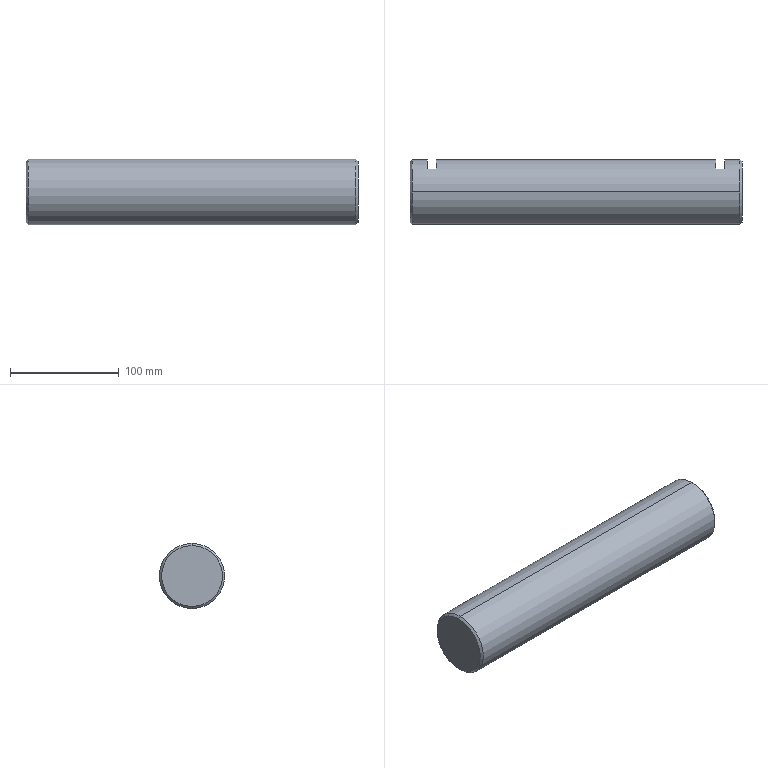Part | STEP file | 04-Driven shaft 1 | 1 solid | 14 faces | box 305 x 60 x 60 mm | volume 857375 mm3 | plane 8 | cone 4 | cylinder 2 | commonest cylinder face diameters 60 x2
STEP:
#1=CARTESIAN_POINT('',(0.,0.,0.));
#2=DIRECTION('',(0.,0.,1.));
#3=DIRECTION('',(1.,0.,0.));
#4=AXIS2_PLACEMENT_3D('',#1,#2,#3);
#5=CARTESIAN_POINT('',(305.,0.,-28.));
#6=VERTEX_POINT('',#5);
#7=CARTESIAN_POINT('',(305.,0.,28.));
#8=VERTEX_POINT('',#7);
#9=CARTESIAN_POINT('',(305.,0.,0.));
#10=DIRECTION('',(1.,0.,0.));
#11=DIRECTION('',(0.,0.,1.));
#12=AXIS2_PLACEMENT_3D('',#9,#10,#11);
#13=CIRCLE('',#12,28.);
#14=CARTESIAN_POINT('',(303.,0.,0.));
#15=DIRECTION('',(-1.,0.,0.));
#16=DIRECTION('',(0.,0.,1.));
#17=AXIS2_PLACEMENT_3D('',#14,#15,#16);
#18=CONICAL_SURFACE('',#17,30.,0.7854);
#19=CARTESIAN_POINT('',(6.283,-2.));
#20=DIRECTION('',(-1.,0.));
#21=VECTOR('',#20,1.);
#22=LINE('',#19,#21);
#23=(GEOMETRIC_REPRESENTATION_CONTEXT(2)PARAMETRIC_REPRESENTATION_CONTEXT()REPRESENTATION_CONTEXT('',''));
#24=DEFINITIONAL_REPRESENTATION('',(#22),#23);
#25=PCURVE('',#18,#24);
#26=CARTESIAN_POINT('',(305.,30.,0.));
#27=DIRECTION('',(-1.,0.,0.));
#28=DIRECTION('',(0.,0.,1.));
#29=AXIS2_PLACEMENT_3D('',#26,#27,#28);
#30=PLANE('',#29);
#31=CARTESIAN_POINT('',(28.,-30.));
#32=CARTESIAN_POINT('',(28.,-78.497));
#33=CARTESIAN_POINT('',(-14.,-54.249));
#34=CARTESIAN_POINT('',(-56.,-30.));
#35=CARTESIAN_POINT('',(-14.,-5.751));
#36=CARTESIAN_POINT('',(28.,18.497));
#37=CARTESIAN_POINT('',(28.,-30.));
#38=(BOUNDED_CURVE()B_SPLINE_CURVE(2,(#31,#32,#33,#34,#35,#36,#37),.UNSPECIFIED.,.T.,.F.)B_SPLINE_CURVE_WITH_KNOTS((1,2,2,2,2,1),(-2.094,0.,2.094,4.189,6.283,8.378),.UNSPECIFIED.)CURVE()GEOMETRIC_REPRESENTATION_ITEM()RATIONAL_B_SPLINE_CURVE((1.,0.5,1.,0.5,1.,0.5,1.))REPRESENTATION_ITEM(''));
#39=(GEOMETRIC_REPRESENTATION_CONTEXT(2)PARAMETRIC_REPRESENTATION_CONTEXT()REPRESENTATION_CONTEXT('',''));
#40=DEFINITIONAL_REPRESENTATION('',(#38),#39);
#41=PCURVE('',#30,#40);
#42=SURFACE_CURVE('',#13,(#25,#41),.PCURVE_S1.);
#43=EDGE_CURVE('',#6,#8,#42,.T.);
#44=ORIENTED_EDGE('',*,*,#43,.F.);
#45=CARTESIAN_POINT('',(303.,0.,-30.));
#46=VERTEX_POINT('',#45);
#47=CARTESIAN_POINT('',(303.,0.,-30.));
#48=DIRECTION('',(-0.7071,0.,-0.7071));
#49=VECTOR('',#48,1.);
#50=LINE('',#47,#49);
#51=CARTESIAN_POINT('',(3.142,0.));
#52=DIRECTION('',(0.,1.));
#53=VECTOR('',#52,1.);
#54=LINE('',#51,#53);
#55=(GEOMETRIC_REPRESENTATION_CONTEXT(2)PARAMETRIC_REPRESENTATION_CONTEXT()REPRESENTATION_CONTEXT('',''));
#56=DEFINITIONAL_REPRESENTATION('',(#54),#55);
#57=PCURVE('',#18,#56);
#58=CARTESIAN_POINT('',(303.,0.,0.));
#59=DIRECTION('',(-1.,0.,0.));
#60=DIRECTION('',(0.,0.,1.));
#61=AXIS2_PLACEMENT_3D('',#58,#59,#60);
#62=CONICAL_SURFACE('',#61,30.,0.7854);
#63=CARTESIAN_POINT('',(3.142,0.));
#64=DIRECTION('',(0.,1.));
#65=VECTOR('',#64,1.);
#66=LINE('',#63,#65);
#67=(GEOMETRIC_REPRESENTATION_CONTEXT(2)PARAMETRIC_REPRESENTATION_CONTEXT()REPRESENTATION_CONTEXT('',''));
#68=DEFINITIONAL_REPRESENTATION('',(#66),#67);
#69=PCURVE('',#62,#68);
#70=SURFACE_CURVE('',#50,(#57,#69),.PCURVE_S1.);
#71=EDGE_CURVE('',#6,#46,#70,.T.);
#72=ORIENTED_EDGE('',*,*,#71,.T.);
#73=CARTESIAN_POINT('',(303.,0.,30.));
#74=VERTEX_POINT('',#73);
#75=CARTESIAN_POINT('',(303.,0.,0.));
#76=DIRECTION('',(-1.,0.,0.));
#77=DIRECTION('',(0.,0.,1.));
#78=AXIS2_PLACEMENT_3D('',#75,#76,#77);
#79=CIRCLE('',#78,30.);
#80=CARTESIAN_POINT('',(0.,0.));
#81=DIRECTION('',(1.,0.));
#82=VECTOR('',#81,1.);
#83=LINE('',#80,#82);
#84=(GEOMETRIC_REPRESENTATION_CONTEXT(2)PARAMETRIC_REPRESENTATION_CONTEXT()REPRESENTATION_CONTEXT('',''));
#85=DEFINITIONAL_REPRESENTATION('',(#83),#84);
#86=PCURVE('',#18,#85);
#87=CARTESIAN_POINT('',(0.,0.,0.));
#88=DIRECTION('',(-1.,0.,0.));
#89=DIRECTION('',(0.,0.,1.));
#90=AXIS2_PLACEMENT_3D('',#87,#88,#89);
#91=CYLINDRICAL_SURFACE('',#90,30.);
#92=CARTESIAN_POINT('',(0.,-303.));
#93=DIRECTION('',(1.,0.));
#94=VECTOR('',#93,1.);
#95=LINE('',#92,#94);
#96=(GEOMETRIC_REPRESENTATION_CONTEXT(2)PARAMETRIC_REPRESENTATION_CONTEXT()REPRESENTATION_CONTEXT('',''));
#97=DEFINITIONAL_REPRESENTATION('',(#95),#96);
#98=PCURVE('',#91,#97);
#99=SURFACE_CURVE('',#79,(#86,#98),.PCURVE_S1.);
#100=EDGE_CURVE('',#74,#46,#99,.T.);
#101=ORIENTED_EDGE('',*,*,#100,.F.);
#102=CARTESIAN_POINT('',(303.,0.,30.));
#103=DIRECTION('',(-0.7071,0.,0.7071));
#104=VECTOR('',#103,1.);
#105=LINE('',#102,#104);
#106=CARTESIAN_POINT('',(0.,0.));
#107=DIRECTION('',(0.,1.));
#108=VECTOR('',#107,1.);
#109=LINE('',#106,#108);
#110=(GEOMETRIC_REPRESENTATION_CONTEXT(2)PARAMETRIC_REPRESENTATION_CONTEXT()REPRESENTATION_CONTEXT('',''));
#111=DEFINITIONAL_REPRESENTATION('',(#109),#110);
#112=PCURVE('',#18,#111);
#113=CARTESIAN_POINT('',(6.283,0.));
#114=DIRECTION('',(0.,1.));
#115=VECTOR('',#114,1.);
#116=LINE('',#113,#115);
#117=(GEOMETRIC_REPRESENTATION_CONTEXT(2)PARAMETRIC_REPRESENTATION_CONTEXT()REPRESENTATION_CONTEXT('',''));
#118=DEFINITIONAL_REPRESENTATION('',(#116),#117);
#119=PCURVE('',#62,#118);
#120=SURFACE_CURVE('',#105,(#112,#119),.PCURVE_S1.);
#121=EDGE_CURVE('',#8,#74,#120,.T.);
#122=ORIENTED_EDGE('',*,*,#121,.F.);
#123=EDGE_LOOP('',(#44,#72,#101,#122));
#124=FACE_BOUND('',#123,.T.);
#125=ADVANCED_FACE('',(#124),#18,.T.);
#126=CARTESIAN_POINT('',(0.,0.,28.));
#127=VERTEX_POINT('',#126);
#128=CARTESIAN_POINT('',(0.,0.,-28.));
#129=VERTEX_POINT('',#128);
#130=CARTESIAN_POINT('',(0.,0.,0.));
#131=DIRECTION('',(-1.,0.,0.));
#132=DIRECTION('',(0.,0.,-1.));
#133=AXIS2_PLACEMENT_3D('',#130,#131,#132);
#134=CIRCLE('',#133,28.);
#135=CARTESIAN_POINT('',(0.,0.,0.));
#136=DIRECTION('',(1.,0.,0.));
#137=DIRECTION('',(0.,0.,-1.));
#138=AXIS2_PLACEMENT_3D('',#135,#136,#137);
#139=CONICAL_SURFACE('',#138,28.,0.7854);
#140=CARTESIAN_POINT('',(6.283,0.));
#141=DIRECTION('',(-1.,0.));
#142=VECTOR('',#141,1.);
#143=LINE('',#140,#142);
#144=(GEOMETRIC_REPRESENTATION_CONTEXT(2)PARAMETRIC_REPRESENTATION_CONTEXT()REPRESENTATION_CONTEXT('',''));
#145=DEFINITIONAL_REPRESENTATION('',(#143),#144);
#146=PCURVE('',#139,#145);
#147=CARTESIAN_POINT('',(0.,0.,0.));
#148=DIRECTION('',(1.,0.,0.));
#149=DIRECTION('',(0.,0.,-1.));
#150=AXIS2_PLACEMENT_3D('',#147,#148,#149);
#151=PLANE('',#150);
#152=CARTESIAN_POINT('',(28.,0.));
#153=CARTESIAN_POINT('',(28.,-48.497));
#154=CARTESIAN_POINT('',(-14.,-24.249));
#155=CARTESIAN_POINT('',(-56.,0.));
#156=CARTESIAN_POINT('',(-14.,24.249));
#157=CARTESIAN_POINT('',(28.,48.497));
#158=CARTESIAN_POINT('',(28.,0.));
#159=(BOUNDED_CURVE()B_SPLINE_CURVE(2,(#152,#153,#154,#155,#156,#157,#158),.UNSPECIFIED.,.T.,.F.)B_SPLINE_CURVE_WITH_KNOTS((1,2,2,2,2,1),(-2.094,0.,2.094,4.189,6.283,8.378),.UNSPECIFIED.)CURVE()GEOMETRIC_REPRESENTATION_ITEM()RATIONAL_B_SPLINE_CURVE((1.,0.5,1.,0.5,1.,0.5,1.))REPRESENTATION_ITEM(''));
#160=(GEOMETRIC_REPRESENTATION_CONTEXT(2)PARAMETRIC_REPRESENTATION_CONTEXT()REPRESENTATION_CONTEXT('',''));
#161=DEFINITIONAL_REPRESENTATION('',(#159),#160);
#162=PCURVE('',#151,#161);
#163=SURFACE_CURVE('',#134,(#146,#162),.PCURVE_S1.);
#164=EDGE_CURVE('',#127,#129,#163,.T.);
#165=ORIENTED_EDGE('',*,*,#164,.F.);
#166=CARTESIAN_POINT('',(2.,0.,30.));
#167=VERTEX_POINT('',#166);
#168=CARTESIAN_POINT('',(0.,0.,28.));
#169=DIRECTION('',(0.7071,0.,0.7071));
#170=VECTOR('',#169,1.);
#171=LINE('',#168,#170);
#172=CARTESIAN_POINT('',(3.142,0.));
#173=DIRECTION('',(0.,1.));
#174=VECTOR('',#173,1.);
#175=LINE('',#172,#174);
#176=(GEOMETRIC_REPRESENTATION_CONTEXT(2)PARAMETRIC_REPRESENTATION_CONTEXT()REPRESENTATION_CONTEXT('',''));
#177=DEFINITIONAL_REPRESENTATION('',(#175),#176);
#178=PCURVE('',#139,#177);
#179=CARTESIAN_POINT('',(0.,0.,0.));
#180=DIRECTION('',(1.,0.,0.));
#181=DIRECTION('',(0.,0.,-1.));
#182=AXIS2_PLACEMENT_3D('',#179,#180,#181);
#183=CONICAL_SURFACE('',#182,28.,0.7854);
#184=CARTESIAN_POINT('',(3.142,0.));
#185=DIRECTION('',(0.,1.));
#186=VECTOR('',#185,1.);
#187=LINE('',#184,#186);
#188=(GEOMETRIC_REPRESENTATION_CONTEXT(2)PARAMETRIC_REPRESENTATION_CONTEXT()REPRESENTATION_CONTEXT('',''));
#189=DEFINITIONAL_REPRESENTATION('',(#187),#188);
#190=PCURVE('',#183,#189);
#191=SURFACE_CURVE('',#171,(#178,#190),.PCURVE_S1.);
#192=EDGE_CURVE('',#127,#167,#191,.T.);
#193=ORIENTED_EDGE('',*,*,#192,.T.);
#194=CARTESIAN_POINT('',(2.,0.,-30.));
#195=VERTEX_POINT('',#194);
#196=CARTESIAN_POINT('',(2.,0.,0.));
#197=DIRECTION('',(1.,0.,0.));
#198=DIRECTION('',(0.,0.,-1.));
#199=AXIS2_PLACEMENT_3D('',#196,#197,#198);
#200=CIRCLE('',#199,30.);
#201=CARTESIAN_POINT('',(0.,2.));
#202=DIRECTION('',(1.,0.));
#203=VECTOR('',#202,1.);
#204=LINE('',#201,#203);
#205=(GEOMETRIC_REPRESENTATION_CONTEXT(2)PARAMETRIC_REPRESENTATION_CONTEXT()REPRESENTATION_CONTEXT('',''));
#206=DEFINITIONAL_REPRESENTATION('',(#204),#205);
#207=PCURVE('',#139,#206);
#208=CARTESIAN_POINT('',(3.142,-2.));
#209=DIRECTION('',(-1.,0.));
#210=VECTOR('',#209,1.);
#211=LINE('',#208,#210);
#212=(GEOMETRIC_REPRESENTATION_CONTEXT(2)PARAMETRIC_REPRESENTATION_CONTEXT()REPRESENTATION_CONTEXT('',''));
#213=DEFINITIONAL_REPRESENTATION('',(#211),#212);
#214=PCURVE('',#91,#213);
#215=SURFACE_CURVE('',#200,(#207,#214),.PCURVE_S1.);
#216=EDGE_CURVE('',#195,#167,#215,.T.);
#217=ORIENTED_EDGE('',*,*,#216,.F.);
#218=CARTESIAN_POINT('',(0.,0.,-28.));
#219=DIRECTION('',(0.7071,0.,-0.7071));
#220=VECTOR('',#219,1.);
#221=LINE('',#218,#220);
#222=CARTESIAN_POINT('',(0.,0.));
#223=DIRECTION('',(0.,1.));
#224=VECTOR('',#223,1.);
#225=LINE('',#222,#224);
#226=(GEOMETRIC_REPRESENTATION_CONTEXT(2)PARAMETRIC_REPRESENTATION_CONTEXT()REPRESENTATION_CONTEXT('',''));
#227=DEFINITIONAL_REPRESENTATION('',(#225),#226);
#228=PCURVE('',#139,#227);
#229=CARTESIAN_POINT('',(6.283,0.));
#230=DIRECTION('',(0.,1.));
#231=VECTOR('',#230,1.);
#232=LINE('',#229,#231);
#233=(GEOMETRIC_REPRESENTATION_CONTEXT(2)PARAMETRIC_REPRESENTATION_CONTEXT()REPRESENTATION_CONTEXT('',''));
#234=DEFINITIONAL_REPRESENTATION('',(#232),#233);
#235=PCURVE('',#183,#234);
#236=SURFACE_CURVE('',#221,(#228,#235),.PCURVE_S1.);
#237=EDGE_CURVE('',#129,#195,#236,.T.);
#238=ORIENTED_EDGE('',*,*,#237,.F.);
#239=EDGE_LOOP('',(#165,#193,#217,#238));
#240=FACE_BOUND('',#239,.T.);
#241=ADVANCED_FACE('',(#240),#139,.T.);
#242=CARTESIAN_POINT('',(24.,21.,-21.424));
#243=VERTEX_POINT('',#242);
#244=CARTESIAN_POINT('',(16.,21.,-21.424));
#245=VERTEX_POINT('',#244);
#246=CARTESIAN_POINT('',(0.,21.,-21.424));
#247=DIRECTION('',(-1.,0.,0.));
#248=VECTOR('',#247,1.);
#249=LINE('',#246,#248);
#250=CARTESIAN_POINT('',(2.366,0.));
#251=DIRECTION('',(0.,1.));
#252=VECTOR('',#251,1.);
#253=LINE('',#250,#252);
#254=(GEOMETRIC_REPRESENTATION_CONTEXT(2)PARAMETRIC_REPRESENTATION_CONTEXT()REPRESENTATION_CONTEXT('',''));
#255=DEFINITIONAL_REPRESENTATION('',(#253),#254);
#256=PCURVE('',#91,#255);
#257=CARTESIAN_POINT('',(0.,21.,0.));
#258=DIRECTION('',(0.,1.,0.));
#259=DIRECTION('',(0.,0.,1.));
#260=AXIS2_PLACEMENT_3D('',#257,#258,#259);
#261=PLANE('',#260);
#262=CARTESIAN_POINT('',(-21.424,0.));
#263=DIRECTION('',(0.,-1.));
#264=VECTOR('',#263,1.);
#265=LINE('',#262,#264);
#266=(GEOMETRIC_REPRESENTATION_CONTEXT(2)PARAMETRIC_REPRESENTATION_CONTEXT()REPRESENTATION_CONTEXT('',''));
#267=DEFINITIONAL_REPRESENTATION('',(#265),#266);
#268=PCURVE('',#261,#267);
#269=SURFACE_CURVE('',#249,(#256,#268),.PCURVE_S1.);
#270=EDGE_CURVE('',#243,#245,#269,.T.);
#271=ORIENTED_EDGE('',*,*,#270,.F.);
#272=CARTESIAN_POINT('',(24.,21.,21.424));
#273=VERTEX_POINT('',#272);
#274=CARTESIAN_POINT('',(24.,0.,0.));
#275=DIRECTION('',(-1.,0.,0.));
#276=DIRECTION('',(0.,0.,1.));
#277=AXIS2_PLACEMENT_3D('',#274,#275,#276);
#278=CIRCLE('',#277,30.);
#279=CARTESIAN_POINT('',(0.,-24.));
#280=DIRECTION('',(1.,0.));
#281=VECTOR('',#280,1.);
#282=LINE('',#279,#281);
#283=(GEOMETRIC_REPRESENTATION_CONTEXT(2)PARAMETRIC_REPRESENTATION_CONTEXT()REPRESENTATION_CONTEXT('',''));
#284=DEFINITIONAL_REPRESENTATION('',(#282),#283);
#285=PCURVE('',#91,#284);
#286=CARTESIAN_POINT('',(24.,31.,-45.622));
#287=DIRECTION('',(-1.,0.,0.));
#288=DIRECTION('',(0.,0.,1.));
#289=AXIS2_PLACEMENT_3D('',#286,#287,#288);
#290=PLANE('',#289);
#291=CARTESIAN_POINT('',(45.622,-31.));
#292=DIRECTION('',(1.,0.));
#293=AXIS2_PLACEMENT_2D('',#291,#292);
#294=CIRCLE('',#293,30.);
#295=(GEOMETRIC_REPRESENTATION_CONTEXT(2)PARAMETRIC_REPRESENTATION_CONTEXT()REPRESENTATION_CONTEXT('',''));
#296=DEFINITIONAL_REPRESENTATION('',(#294),#295);
#297=PCURVE('',#290,#296);
#298=SURFACE_CURVE('',#278,(#285,#297),.PCURVE_S1.);
#299=EDGE_CURVE('',#273,#243,#298,.T.);
#300=ORIENTED_EDGE('',*,*,#299,.F.);
#301=CARTESIAN_POINT('',(16.,21.,21.424));
#302=VERTEX_POINT('',#301);
#303=CARTESIAN_POINT('',(0.,21.,21.424));
#304=DIRECTION('',(1.,0.,0.));
#305=VECTOR('',#304,1.);
#306=LINE('',#303,#305);
#307=CARTESIAN_POINT('',(0.7754,0.));
#308=DIRECTION('',(0.,-1.));
#309=VECTOR('',#308,1.);
#310=LINE('',#307,#309);
#311=(GEOMETRIC_REPRESENTATION_CONTEXT(2)PARAMETRIC_REPRESENTATION_CONTEXT()REPRESENTATION_CONTEXT('',''));
#312=DEFINITIONAL_REPRESENTATION('',(#310),#311);
#313=PCURVE('',#91,#312);
#314=CARTESIAN_POINT('',(21.424,0.));
#315=DIRECTION('',(0.,1.));
#316=VECTOR('',#315,1.);
#317=LINE('',#314,#316);
#318=(GEOMETRIC_REPRESENTATION_CONTEXT(2)PARAMETRIC_REPRESENTATION_CONTEXT()REPRESENTATION_CONTEXT('',''));
#319=DEFINITIONAL_REPRESENTATION('',(#317),#318);
#320=PCURVE('',#261,#319);
#321=SURFACE_CURVE('',#306,(#313,#320),.PCURVE_S1.);
#322=EDGE_CURVE('',#302,#273,#321,.T.);
#323=ORIENTED_EDGE('',*,*,#322,.F.);
#324=CARTESIAN_POINT('',(16.,0.,0.));
#325=DIRECTION('',(1.,0.,0.));
#326=DIRECTION('',(0.,0.,-1.));
#327=AXIS2_PLACEMENT_3D('',#324,#325,#326);
#328=CIRCLE('',#327,30.);
#329=CARTESIAN_POINT('',(3.142,-16.));
#330=DIRECTION('',(-1.,0.));
#331=VECTOR('',#330,1.);
#332=LINE('',#329,#331);
#333=(GEOMETRIC_REPRESENTATION_CONTEXT(2)PARAMETRIC_REPRESENTATION_CONTEXT()REPRESENTATION_CONTEXT('',''));
#334=DEFINITIONAL_REPRESENTATION('',(#332),#333);
#335=PCURVE('',#91,#334);
#336=CARTESIAN_POINT('',(16.,31.,-45.622));
#337=DIRECTION('',(1.,0.,0.));
#338=DIRECTION('',(0.,0.,-1.));
#339=AXIS2_PLACEMENT_3D('',#336,#337,#338);
#340=PLANE('',#339);
#341=CARTESIAN_POINT('',(-45.622,-31.));
#342=DIRECTION('',(1.,0.));
#343=AXIS2_PLACEMENT_2D('',#341,#342);
#344=CIRCLE('',#343,30.);
#345=(GEOMETRIC_REPRESENTATION_CONTEXT(2)PARAMETRIC_REPRESENTATION_CONTEXT()REPRESENTATION_CONTEXT('',''));
#346=DEFINITIONAL_REPRESENTATION('',(#344),#345);
#347=PCURVE('',#340,#346);
#348=SURFACE_CURVE('',#328,(#335,#347),.PCURVE_S1.);
#349=EDGE_CURVE('',#245,#302,#348,.T.);
#350=ORIENTED_EDGE('',*,*,#349,.F.);
#351=EDGE_LOOP('',(#271,#300,#323,#350));
#352=FACE_BOUND('',#351,.T.);
#353=CARTESIAN_POINT('',(289.,21.,-21.424));
#354=VERTEX_POINT('',#353);
#355=CARTESIAN_POINT('',(281.,21.,-21.424));
#356=VERTEX_POINT('',#355);
#357=CARTESIAN_POINT('',(0.,21.,-21.424));
#358=DIRECTION('',(-1.,0.,0.));
#359=VECTOR('',#358,1.);
#360=LINE('',#357,#359);
#361=CARTESIAN_POINT('',(2.366,0.));
#362=DIRECTION('',(0.,1.));
#363=VECTOR('',#362,1.);
#364=LINE('',#361,#363);
#365=(GEOMETRIC_REPRESENTATION_CONTEXT(2)PARAMETRIC_REPRESENTATION_CONTEXT()REPRESENTATION_CONTEXT('',''));
#366=DEFINITIONAL_REPRESENTATION('',(#364),#365);
#367=PCURVE('',#91,#366);
#368=CARTESIAN_POINT('',(0.,21.,0.));
#369=DIRECTION('',(0.,1.,0.));
#370=DIRECTION('',(0.,0.,1.));
#371=AXIS2_PLACEMENT_3D('',#368,#369,#370);
#372=PLANE('',#371);
#373=CARTESIAN_POINT('',(-21.424,0.));
#374=DIRECTION('',(0.,-1.));
#375=VECTOR('',#374,1.);
#376=LINE('',#373,#375);
#377=(GEOMETRIC_REPRESENTATION_CONTEXT(2)PARAMETRIC_REPRESENTATION_CONTEXT()REPRESENTATION_CONTEXT('',''));
#378=DEFINITIONAL_REPRESENTATION('',(#376),#377);
#379=PCURVE('',#372,#378);
#380=SURFACE_CURVE('',#360,(#367,#379),.PCURVE_S1.);
#381=EDGE_CURVE('',#354,#356,#380,.T.);
#382=ORIENTED_EDGE('',*,*,#381,.F.);
#383=CARTESIAN_POINT('',(289.,21.,21.424));
#384=VERTEX_POINT('',#383);
#385=CARTESIAN_POINT('',(289.,0.,0.));
#386=DIRECTION('',(-1.,0.,0.));
#387=DIRECTION('',(0.,0.,1.));
#388=AXIS2_PLACEMENT_3D('',#385,#386,#387);
#389=CIRCLE('',#388,30.);
#390=CARTESIAN_POINT('',(0.,-289.));
#391=DIRECTION('',(1.,0.));
#392=VECTOR('',#391,1.);
#393=LINE('',#390,#392);
#394=(GEOMETRIC_REPRESENTATION_CONTEXT(2)PARAMETRIC_REPRESENTATION_CONTEXT()REPRESENTATION_CONTEXT('',''));
#395=DEFINITIONAL_REPRESENTATION('',(#393),#394);
#396=PCURVE('',#91,#395);
#397=CARTESIAN_POINT('',(289.,31.,-54.746));
#398=DIRECTION('',(-1.,0.,0.));
#399=DIRECTION('',(0.,0.,1.));
#400=AXIS2_PLACEMENT_3D('',#397,#398,#399);
#401=PLANE('',#400);
#402=CARTESIAN_POINT('',(54.746,-31.));
#403=DIRECTION('',(1.,0.));
#404=AXIS2_PLACEMENT_2D('',#402,#403);
#405=CIRCLE('',#404,30.);
#406=(GEOMETRIC_REPRESENTATION_CONTEXT(2)PARAMETRIC_REPRESENTATION_CONTEXT()REPRESENTATION_CONTEXT('',''));
#407=DEFINITIONAL_REPRESENTATION('',(#405),#406);
#408=PCURVE('',#401,#407);
#409=SURFACE_CURVE('',#389,(#396,#408),.PCURVE_S1.);
#410=EDGE_CURVE('',#384,#354,#409,.T.);
#411=ORIENTED_EDGE('',*,*,#410,.F.);
#412=CARTESIAN_POINT('',(281.,21.,21.424));
#413=VERTEX_POINT('',#412);
#414=CARTESIAN_POINT('',(0.,21.,21.424));
#415=DIRECTION('',(1.,0.,0.));
#416=VECTOR('',#415,1.);
#417=LINE('',#414,#416);
#418=CARTESIAN_POINT('',(0.7754,0.));
#419=DIRECTION('',(0.,-1.));
#420=VECTOR('',#419,1.);
#421=LINE('',#418,#420);
#422=(GEOMETRIC_REPRESENTATION_CONTEXT(2)PARAMETRIC_REPRESENTATION_CONTEXT()REPRESENTATION_CONTEXT('',''));
#423=DEFINITIONAL_REPRESENTATION('',(#421),#422);
#424=PCURVE('',#91,#423);
#425=CARTESIAN_POINT('',(21.424,0.));
#426=DIRECTION('',(0.,1.));
#427=VECTOR('',#426,1.);
#428=LINE('',#425,#427);
#429=(GEOMETRIC_REPRESENTATION_CONTEXT(2)PARAMETRIC_REPRESENTATION_CONTEXT()REPRESENTATION_CONTEXT('',''));
#430=DEFINITIONAL_REPRESENTATION('',(#428),#429);
#431=PCURVE('',#372,#430);
#432=SURFACE_CURVE('',#417,(#424,#431),.PCURVE_S1.);
#433=EDGE_CURVE('',#413,#384,#432,.T.);
#434=ORIENTED_EDGE('',*,*,#433,.F.);
#435=CARTESIAN_POINT('',(281.,0.,0.));
#436=DIRECTION('',(1.,0.,0.));
#437=DIRECTION('',(0.,0.,-1.));
#438=AXIS2_PLACEMENT_3D('',#435,#436,#437);
#439=CIRCLE('',#438,30.);
#440=CARTESIAN_POINT('',(3.142,-281.));
#441=DIRECTION('',(-1.,0.));
#442=VECTOR('',#441,1.);
#443=LINE('',#440,#442);
#444=(GEOMETRIC_REPRESENTATION_CONTEXT(2)PARAMETRIC_REPRESENTATION_CONTEXT()REPRESENTATION_CONTEXT('',''));
#445=DEFINITIONAL_REPRESENTATION('',(#443),#444);
#446=PCURVE('',#91,#445);
#447=CARTESIAN_POINT('',(281.,31.,-54.746));
#448=DIRECTION('',(1.,0.,0.));
#449=DIRECTION('',(0.,0.,-1.));
#450=AXIS2_PLACEMENT_3D('',#447,#448,#449);
#451=PLANE('',#450);
#452=CARTESIAN_POINT('',(-54.746,-31.));
#453=DIRECTION('',(1.,0.));
#454=AXIS2_PLACEMENT_2D('',#452,#453);
#455=CIRCLE('',#454,30.);
#456=(GEOMETRIC_REPRESENTATION_CONTEXT(2)PARAMETRIC_REPRESENTATION_CONTEXT()REPRESENTATION_CONTEXT('',''));
#457=DEFINITIONAL_REPRESENTATION('',(#455),#456);
#458=PCURVE('',#451,#457);
#459=SURFACE_CURVE('',#439,(#446,#458),.PCURVE_S1.);
#460=EDGE_CURVE('',#356,#413,#459,.T.);
#461=ORIENTED_EDGE('',*,*,#460,.F.);
#462=EDGE_LOOP('',(#382,#411,#434,#461));
#463=FACE_BOUND('',#462,.T.);
#464=ORIENTED_EDGE('',*,*,#100,.T.);
#465=CARTESIAN_POINT('',(0.,0.,-30.));
#466=DIRECTION('',(-1.,0.,0.));
#467=VECTOR('',#466,1.);
#468=LINE('',#465,#467);
#469=CARTESIAN_POINT('',(3.142,0.));
#470=DIRECTION('',(0.,1.));
#471=VECTOR('',#470,1.);
#472=LINE('',#469,#471);
#473=(GEOMETRIC_REPRESENTATION_CONTEXT(2)PARAMETRIC_REPRESENTATION_CONTEXT()REPRESENTATION_CONTEXT('',''));
#474=DEFINITIONAL_REPRESENTATION('',(#472),#473);
#475=PCURVE('',#91,#474);
#476=CARTESIAN_POINT('',(0.,0.,0.));
#477=DIRECTION('',(-1.,0.,0.));
#478=DIRECTION('',(0.,0.,1.));
#479=AXIS2_PLACEMENT_3D('',#476,#477,#478);
#480=CYLINDRICAL_SURFACE('',#479,30.);
#481=CARTESIAN_POINT('',(3.142,0.));
#482=DIRECTION('',(0.,1.));
#483=VECTOR('',#482,1.);
#484=LINE('',#481,#483);
#485=(GEOMETRIC_REPRESENTATION_CONTEXT(2)PARAMETRIC_REPRESENTATION_CONTEXT()REPRESENTATION_CONTEXT('',''));
#486=DEFINITIONAL_REPRESENTATION('',(#484),#485);
#487=PCURVE('',#480,#486);
#488=SURFACE_CURVE('',#468,(#475,#487),.PCURVE_S1.);
#489=EDGE_CURVE('',#46,#195,#488,.T.);
#490=ORIENTED_EDGE('',*,*,#489,.T.);
#491=ORIENTED_EDGE('',*,*,#216,.T.);
#492=CARTESIAN_POINT('',(0.,0.,30.));
#493=DIRECTION('',(-1.,0.,0.));
#494=VECTOR('',#493,1.);
#495=LINE('',#492,#494);
#496=CARTESIAN_POINT('',(0.,0.));
#497=DIRECTION('',(0.,1.));
#498=VECTOR('',#497,1.);
#499=LINE('',#496,#498);
#500=(GEOMETRIC_REPRESENTATION_CONTEXT(2)PARAMETRIC_REPRESENTATION_CONTEXT()REPRESENTATION_CONTEXT('',''));
#501=DEFINITIONAL_REPRESENTATION('',(#499),#500);
#502=PCURVE('',#91,#501);
#503=CARTESIAN_POINT('',(6.283,0.));
#504=DIRECTION('',(0.,1.));
#505=VECTOR('',#504,1.);
#506=LINE('',#503,#505);
#507=(GEOMETRIC_REPRESENTATION_CONTEXT(2)PARAMETRIC_REPRESENTATION_CONTEXT()REPRESENTATION_CONTEXT('',''));
#508=DEFINITIONAL_REPRESENTATION('',(#506),#507);
#509=PCURVE('',#480,#508);
#510=SURFACE_CURVE('',#495,(#502,#509),.PCURVE_S1.);
#511=EDGE_CURVE('',#74,#167,#510,.T.);
#512=ORIENTED_EDGE('',*,*,#511,.F.);
#513=EDGE_LOOP('',(#464,#490,#491,#512));
#514=FACE_BOUND('',#513,.T.);
#515=ADVANCED_FACE('',(#352,#463,#514),#91,.T.);
#516=ORIENTED_EDGE('',*,*,#489,.F.);
#517=CARTESIAN_POINT('',(303.,0.,0.));
#518=DIRECTION('',(-1.,0.,0.));
#519=DIRECTION('',(0.,0.,1.));
#520=AXIS2_PLACEMENT_3D('',#517,#518,#519);
#521=CIRCLE('',#520,30.);
#522=CARTESIAN_POINT('',(0.,-303.));
#523=DIRECTION('',(1.,0.));
#524=VECTOR('',#523,1.);
#525=LINE('',#522,#524);
#526=(GEOMETRIC_REPRESENTATION_CONTEXT(2)PARAMETRIC_REPRESENTATION_CONTEXT()REPRESENTATION_CONTEXT('',''));
#527=DEFINITIONAL_REPRESENTATION('',(#525),#526);
#528=PCURVE('',#480,#527);
#529=CARTESIAN_POINT('',(0.,0.));
#530=DIRECTION('',(1.,0.));
#531=VECTOR('',#530,1.);
#532=LINE('',#529,#531);
#533=(GEOMETRIC_REPRESENTATION_CONTEXT(2)PARAMETRIC_REPRESENTATION_CONTEXT()REPRESENTATION_CONTEXT('',''));
#534=DEFINITIONAL_REPRESENTATION('',(#532),#533);
#535=PCURVE('',#62,#534);
#536=SURFACE_CURVE('',#521,(#528,#535),.PCURVE_S1.);
#537=EDGE_CURVE('',#46,#74,#536,.T.);
#538=ORIENTED_EDGE('',*,*,#537,.T.);
#539=ORIENTED_EDGE('',*,*,#511,.T.);
#540=CARTESIAN_POINT('',(2.,0.,0.));
#541=DIRECTION('',(1.,0.,0.));
#542=DIRECTION('',(0.,0.,-1.));
#543=AXIS2_PLACEMENT_3D('',#540,#541,#542);
#544=CIRCLE('',#543,30.);
#545=CARTESIAN_POINT('',(9.425,-2.));
#546=DIRECTION('',(-1.,0.));
#547=VECTOR('',#546,1.);
#548=LINE('',#545,#547);
#549=(GEOMETRIC_REPRESENTATION_CONTEXT(2)PARAMETRIC_REPRESENTATION_CONTEXT()REPRESENTATION_CONTEXT('',''));
#550=DEFINITIONAL_REPRESENTATION('',(#548),#549);
#551=PCURVE('',#480,#550);
#552=CARTESIAN_POINT('',(0.,2.));
#553=DIRECTION('',(1.,0.));
#554=VECTOR('',#553,1.);
#555=LINE('',#552,#554);
#556=(GEOMETRIC_REPRESENTATION_CONTEXT(2)PARAMETRIC_REPRESENTATION_CONTEXT()REPRESENTATION_CONTEXT('',''));
#557=DEFINITIONAL_REPRESENTATION('',(#555),#556);
#558=PCURVE('',#183,#557);
#559=SURFACE_CURVE('',#544,(#551,#558),.PCURVE_S1.);
#560=EDGE_CURVE('',#167,#195,#559,.T.);
#561=ORIENTED_EDGE('',*,*,#560,.T.);
#562=EDGE_LOOP('',(#516,#538,#539,#561));
#563=FACE_BOUND('',#562,.T.);
#564=ADVANCED_FACE('',(#563),#480,.T.);
#565=CARTESIAN_POINT('',(0.,0.,0.));
#566=DIRECTION('',(-1.,0.,0.));
#567=DIRECTION('',(0.,0.,-1.));
#568=AXIS2_PLACEMENT_3D('',#565,#566,#567);
#569=CIRCLE('',#568,28.);
#570=CARTESIAN_POINT('',(28.,0.));
#571=CARTESIAN_POINT('',(28.,-48.497));
#572=CARTESIAN_POINT('',(-14.,-24.249));
#573=CARTESIAN_POINT('',(-56.,0.));
#574=CARTESIAN_POINT('',(-14.,24.249));
#575=CARTESIAN_POINT('',(28.,48.497));
#576=CARTESIAN_POINT('',(28.,0.));
#577=(BOUNDED_CURVE()B_SPLINE_CURVE(2,(#570,#571,#572,#573,#574,#575,#576),.UNSPECIFIED.,.T.,.F.)B_SPLINE_CURVE_WITH_KNOTS((1,2,2,2,2,1),(-2.094,0.,2.094,4.189,6.283,8.378),.UNSPECIFIED.)CURVE()GEOMETRIC_REPRESENTATION_ITEM()RATIONAL_B_SPLINE_CURVE((1.,0.5,1.,0.5,1.,0.5,1.))REPRESENTATION_ITEM(''));
#578=(GEOMETRIC_REPRESENTATION_CONTEXT(2)PARAMETRIC_REPRESENTATION_CONTEXT()REPRESENTATION_CONTEXT('',''));
#579=DEFINITIONAL_REPRESENTATION('',(#577),#578);
#580=PCURVE('',#151,#579);
#581=CARTESIAN_POINT('',(6.283,0.));
#582=DIRECTION('',(-1.,0.));
#583=VECTOR('',#582,1.);
#584=LINE('',#581,#583);
#585=(GEOMETRIC_REPRESENTATION_CONTEXT(2)PARAMETRIC_REPRESENTATION_CONTEXT()REPRESENTATION_CONTEXT('',''));
#586=DEFINITIONAL_REPRESENTATION('',(#584),#585);
#587=PCURVE('',#183,#586);
#588=SURFACE_CURVE('',#569,(#580,#587),.PCURVE_S1.);
#589=EDGE_CURVE('',#129,#127,#588,.T.);
#590=ORIENTED_EDGE('',*,*,#589,.T.);
#591=ORIENTED_EDGE('',*,*,#164,.T.);
#592=EDGE_LOOP('',(#590,#591));
#593=FACE_BOUND('',#592,.T.);
#594=ADVANCED_FACE('',(#593),#151,.F.);
#595=CARTESIAN_POINT('',(305.,0.,0.));
#596=DIRECTION('',(1.,0.,0.));
#597=DIRECTION('',(0.,0.,1.));
#598=AXIS2_PLACEMENT_3D('',#595,#596,#597);
#599=CIRCLE('',#598,28.);
#600=CARTESIAN_POINT('',(28.,-30.));
#601=CARTESIAN_POINT('',(28.,-78.497));
#602=CARTESIAN_POINT('',(-14.,-54.249));
#603=CARTESIAN_POINT('',(-56.,-30.));
#604=CARTESIAN_POINT('',(-14.,-5.751));
#605=CARTESIAN_POINT('',(28.,18.497));
#606=CARTESIAN_POINT('',(28.,-30.));
#607=(BOUNDED_CURVE()B_SPLINE_CURVE(2,(#600,#601,#602,#603,#604,#605,#606),.UNSPECIFIED.,.T.,.F.)B_SPLINE_CURVE_WITH_KNOTS((1,2,2,2,2,1),(-2.094,0.,2.094,4.189,6.283,8.378),.UNSPECIFIED.)CURVE()GEOMETRIC_REPRESENTATION_ITEM()RATIONAL_B_SPLINE_CURVE((1.,0.5,1.,0.5,1.,0.5,1.))REPRESENTATION_ITEM(''));
#608=(GEOMETRIC_REPRESENTATION_CONTEXT(2)PARAMETRIC_REPRESENTATION_CONTEXT()REPRESENTATION_CONTEXT('',''));
#609=DEFINITIONAL_REPRESENTATION('',(#607),#608);
#610=PCURVE('',#30,#609);
#611=CARTESIAN_POINT('',(6.283,-2.));
#612=DIRECTION('',(-1.,0.));
#613=VECTOR('',#612,1.);
#614=LINE('',#611,#613);
#615=(GEOMETRIC_REPRESENTATION_CONTEXT(2)PARAMETRIC_REPRESENTATION_CONTEXT()REPRESENTATION_CONTEXT('',''));
#616=DEFINITIONAL_REPRESENTATION('',(#614),#615);
#617=PCURVE('',#62,#616);
#618=SURFACE_CURVE('',#599,(#610,#617),.PCURVE_S1.);
#619=EDGE_CURVE('',#8,#6,#618,.T.);
#620=ORIENTED_EDGE('',*,*,#619,.T.);
#621=ORIENTED_EDGE('',*,*,#43,.T.);
#622=EDGE_LOOP('',(#620,#621));
#623=FACE_BOUND('',#622,.T.);
#624=ADVANCED_FACE('',(#623),#30,.F.);
#625=ORIENTED_EDGE('',*,*,#349,.T.);
#626=CARTESIAN_POINT('',(16.,21.,-45.622));
#627=DIRECTION('',(0.,0.,1.));
#628=VECTOR('',#627,1.);
#629=LINE('',#626,#628);
#630=CARTESIAN_POINT('',(0.,-10.));
#631=DIRECTION('',(-1.,0.));
#632=VECTOR('',#631,1.);
#633=LINE('',#630,#632);
#634=(GEOMETRIC_REPRESENTATION_CONTEXT(2)PARAMETRIC_REPRESENTATION_CONTEXT()REPRESENTATION_CONTEXT('',''));
#635=DEFINITIONAL_REPRESENTATION('',(#633),#634);
#636=PCURVE('',#340,#635);
#637=CARTESIAN_POINT('',(-45.622,16.));
#638=DIRECTION('',(1.,0.));
#639=VECTOR('',#638,1.);
#640=LINE('',#637,#639);
#641=(GEOMETRIC_REPRESENTATION_CONTEXT(2)PARAMETRIC_REPRESENTATION_CONTEXT()REPRESENTATION_CONTEXT('',''));
#642=DEFINITIONAL_REPRESENTATION('',(#640),#641);
#643=PCURVE('',#261,#642);
#644=SURFACE_CURVE('',#629,(#636,#643),.PCURVE_S1.);
#645=EDGE_CURVE('',#245,#302,#644,.T.);
#646=ORIENTED_EDGE('',*,*,#645,.F.);
#647=EDGE_LOOP('',(#625,#646));
#648=FACE_BOUND('',#647,.T.);
#649=ADVANCED_FACE('',(#648),#340,.T.);
#650=ORIENTED_EDGE('',*,*,#299,.T.);
#651=CARTESIAN_POINT('',(24.,21.,-45.622));
#652=DIRECTION('',(0.,0.,-1.));
#653=VECTOR('',#652,1.);
#654=LINE('',#651,#653);
#655=CARTESIAN_POINT('',(0.,-10.));
#656=DIRECTION('',(-1.,0.));
#657=VECTOR('',#656,1.);
#658=LINE('',#655,#657);
#659=(GEOMETRIC_REPRESENTATION_CONTEXT(2)PARAMETRIC_REPRESENTATION_CONTEXT()REPRESENTATION_CONTEXT('',''));
#660=DEFINITIONAL_REPRESENTATION('',(#658),#659);
#661=PCURVE('',#290,#660);
#662=CARTESIAN_POINT('',(-45.622,24.));
#663=DIRECTION('',(-1.,0.));
#664=VECTOR('',#663,1.);
#665=LINE('',#662,#664);
#666=(GEOMETRIC_REPRESENTATION_CONTEXT(2)PARAMETRIC_REPRESENTATION_CONTEXT()REPRESENTATION_CONTEXT('',''));
#667=DEFINITIONAL_REPRESENTATION('',(#665),#666);
#668=PCURVE('',#261,#667);
#669=SURFACE_CURVE('',#654,(#661,#668),.PCURVE_S1.);
#670=EDGE_CURVE('',#273,#243,#669,.T.);
#671=ORIENTED_EDGE('',*,*,#670,.F.);
#672=EDGE_LOOP('',(#650,#671));
#673=FACE_BOUND('',#672,.T.);
#674=ADVANCED_FACE('',(#673),#290,.T.);
#675=ORIENTED_EDGE('',*,*,#270,.T.);
#676=ORIENTED_EDGE('',*,*,#645,.T.);
#677=ORIENTED_EDGE('',*,*,#322,.T.);
#678=ORIENTED_EDGE('',*,*,#670,.T.);
#679=EDGE_LOOP('',(#675,#676,#677,#678));
#680=FACE_BOUND('',#679,.T.);
#681=ADVANCED_FACE('',(#680),#261,.T.);
#682=ORIENTED_EDGE('',*,*,#460,.T.);
#683=CARTESIAN_POINT('',(281.,21.,-54.746));
#684=DIRECTION('',(0.,0.,1.));
#685=VECTOR('',#684,1.);
#686=LINE('',#683,#685);
#687=CARTESIAN_POINT('',(0.,-10.));
#688=DIRECTION('',(-1.,0.));
#689=VECTOR('',#688,1.);
#690=LINE('',#687,#689);
#691=(GEOMETRIC_REPRESENTATION_CONTEXT(2)PARAMETRIC_REPRESENTATION_CONTEXT()REPRESENTATION_CONTEXT('',''));
#692=DEFINITIONAL_REPRESENTATION('',(#690),#691);
#693=PCURVE('',#451,#692);
#694=CARTESIAN_POINT('',(-54.746,281.));
#695=DIRECTION('',(1.,0.));
#696=VECTOR('',#695,1.);
#697=LINE('',#694,#696);
#698=(GEOMETRIC_REPRESENTATION_CONTEXT(2)PARAMETRIC_REPRESENTATION_CONTEXT()REPRESENTATION_CONTEXT('',''));
#699=DEFINITIONAL_REPRESENTATION('',(#697),#698);
#700=PCURVE('',#372,#699);
#701=SURFACE_CURVE('',#686,(#693,#700),.PCURVE_S1.);
#702=EDGE_CURVE('',#356,#413,#701,.T.);
#703=ORIENTED_EDGE('',*,*,#702,.F.);
#704=EDGE_LOOP('',(#682,#703));
#705=FACE_BOUND('',#704,.T.);
#706=ADVANCED_FACE('',(#705),#451,.T.);
#707=ORIENTED_EDGE('',*,*,#410,.T.);
#708=CARTESIAN_POINT('',(289.,21.,-54.746));
#709=DIRECTION('',(0.,0.,-1.));
#710=VECTOR('',#709,1.);
#711=LINE('',#708,#710);
#712=CARTESIAN_POINT('',(0.,-10.));
#713=DIRECTION('',(-1.,0.));
#714=VECTOR('',#713,1.);
#715=LINE('',#712,#714);
#716=(GEOMETRIC_REPRESENTATION_CONTEXT(2)PARAMETRIC_REPRESENTATION_CONTEXT()REPRESENTATION_CONTEXT('',''));
#717=DEFINITIONAL_REPRESENTATION('',(#715),#716);
#718=PCURVE('',#401,#717);
#719=CARTESIAN_POINT('',(-54.746,289.));
#720=DIRECTION('',(-1.,0.));
#721=VECTOR('',#720,1.);
#722=LINE('',#719,#721);
#723=(GEOMETRIC_REPRESENTATION_CONTEXT(2)PARAMETRIC_REPRESENTATION_CONTEXT()REPRESENTATION_CONTEXT('',''));
#724=DEFINITIONAL_REPRESENTATION('',(#722),#723);
#725=PCURVE('',#372,#724);
#726=SURFACE_CURVE('',#711,(#718,#725),.PCURVE_S1.);
#727=EDGE_CURVE('',#384,#354,#726,.T.);
#728=ORIENTED_EDGE('',*,*,#727,.F.);
#729=EDGE_LOOP('',(#707,#728));
#730=FACE_BOUND('',#729,.T.);
#731=ADVANCED_FACE('',(#730),#401,.T.);
#732=ORIENTED_EDGE('',*,*,#381,.T.);
#733=ORIENTED_EDGE('',*,*,#702,.T.);
#734=ORIENTED_EDGE('',*,*,#433,.T.);
#735=ORIENTED_EDGE('',*,*,#727,.T.);
#736=EDGE_LOOP('',(#732,#733,#734,#735));
#737=FACE_BOUND('',#736,.T.);
#738=ADVANCED_FACE('',(#737),#372,.T.);
#739=ORIENTED_EDGE('',*,*,#192,.F.);
#740=ORIENTED_EDGE('',*,*,#589,.F.);
#741=ORIENTED_EDGE('',*,*,#237,.T.);
#742=ORIENTED_EDGE('',*,*,#560,.F.);
#743=EDGE_LOOP('',(#739,#740,#741,#742));
#744=FACE_BOUND('',#743,.T.);
#745=ADVANCED_FACE('',(#744),#183,.T.);
#746=ORIENTED_EDGE('',*,*,#71,.F.);
#747=ORIENTED_EDGE('',*,*,#619,.F.);
#748=ORIENTED_EDGE('',*,*,#121,.T.);
#749=ORIENTED_EDGE('',*,*,#537,.F.);
#750=EDGE_LOOP('',(#746,#747,#748,#749));
#751=FACE_BOUND('',#750,.T.);
#752=ADVANCED_FACE('',(#751),#62,.T.);
#753=CLOSED_SHELL('',(#125,#241,#515,#564,#594,#624,#649,#674,#681,#706,#731,#738,#745,#752));
#754=MANIFOLD_SOLID_BREP('',#753);
#755=(LENGTH_UNIT()NAMED_UNIT(*)SI_UNIT(.MILLI.,.METRE.));
#756=UNCERTAINTY_MEASURE_WITH_UNIT(LENGTH_MEASURE(0.0000001),#755,'','');
#757=(NAMED_UNIT(*)PLANE_ANGLE_UNIT()SI_UNIT($,.RADIAN.));
#758=(NAMED_UNIT(*)SI_UNIT($,.STERADIAN.)SOLID_ANGLE_UNIT());
#759=(GEOMETRIC_REPRESENTATION_CONTEXT(3)GLOBAL_UNCERTAINTY_ASSIGNED_CONTEXT((#756))GLOBAL_UNIT_ASSIGNED_CONTEXT((#755,#757,#758))REPRESENTATION_CONTEXT('',''));
#760=ADVANCED_BREP_SHAPE_REPRESENTATION('',(#4,#754),#759);